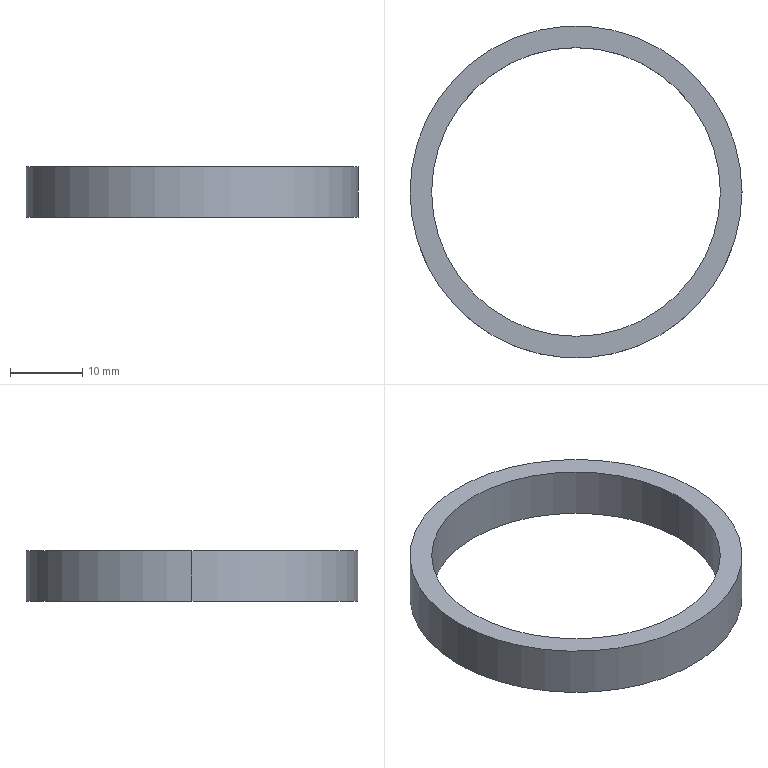Part | SolidWorks | features Extrusion 1 | 1 solid | 6 faces | box 46 x 46 x 7 mm | volume 2837 mm3 | cylinder 4 | plane 2 | commonest cylinder face diameters 40 x2 46 x2
STEP:
#1=CARTESIAN_POINT('',(-20.,0.,7.));
#2=VERTEX_POINT('',#1);
#3=CARTESIAN_POINT('',(20.,0.,7.));
#4=VERTEX_POINT('',#3);
#5=CARTESIAN_POINT('',(0.,0.,7.));
#6=DIRECTION('',(0.,0.,1.));
#7=DIRECTION('',(1.,0.,0.));
#8=AXIS2_PLACEMENT_3D('',#5,#6,#7);
#9=CIRCLE('',#8,20.);
#10=EDGE_CURVE('',#2,#4,#9,.T.);
#11=ORIENTED_EDGE('',*,*,#10,.T.);
#12=CARTESIAN_POINT('',(20.,0.,0.));
#13=VERTEX_POINT('',#12);
#14=CARTESIAN_POINT('',(20.,0.,7.));
#15=DIRECTION('',(0.,0.,-1.));
#16=VECTOR('',#15,1000.);
#17=LINE('',#14,#16);
#18=EDGE_CURVE('',#4,#13,#17,.T.);
#19=ORIENTED_EDGE('',*,*,#18,.T.);
#20=CARTESIAN_POINT('',(-20.,0.,0.));
#21=VERTEX_POINT('',#20);
#22=CARTESIAN_POINT('',(0.,0.,0.));
#23=DIRECTION('',(0.,0.,1.));
#24=DIRECTION('',(1.,0.,0.));
#25=AXIS2_PLACEMENT_3D('',#22,#23,#24);
#26=CIRCLE('',#25,20.);
#27=EDGE_CURVE('',#21,#13,#26,.T.);
#28=ORIENTED_EDGE('',*,*,#27,.F.);
#29=CARTESIAN_POINT('',(-20.,0.,7.));
#30=DIRECTION('',(0.,0.,-1.));
#31=VECTOR('',#30,1000.);
#32=LINE('',#29,#31);
#33=EDGE_CURVE('',#2,#21,#32,.T.);
#34=ORIENTED_EDGE('',*,*,#33,.F.);
#35=EDGE_LOOP('',(#11,#19,#28,#34));
#36=FACE_OUTER_BOUND('',#35,.T.);
#37=CARTESIAN_POINT('',(0.,0.,7.));
#38=DIRECTION('',(0.,0.,-1.));
#39=DIRECTION('',(-1.,0.,0.));
#40=AXIS2_PLACEMENT_3D('',#37,#38,#39);
#41=CYLINDRICAL_SURFACE('',#40,20.);
#42=ADVANCED_FACE('',(#36),#41,.F.);
#43=CARTESIAN_POINT('',(23.,0.,7.));
#44=VERTEX_POINT('',#43);
#45=CARTESIAN_POINT('',(-23.,0.,7.));
#46=VERTEX_POINT('',#45);
#47=CARTESIAN_POINT('',(0.,0.,7.));
#48=DIRECTION('',(0.,0.,1.));
#49=DIRECTION('',(1.,0.,0.));
#50=AXIS2_PLACEMENT_3D('',#47,#48,#49);
#51=CIRCLE('',#50,23.);
#52=EDGE_CURVE('',#44,#46,#51,.T.);
#53=ORIENTED_EDGE('',*,*,#52,.F.);
#54=CARTESIAN_POINT('',(23.,0.,0.));
#55=VERTEX_POINT('',#54);
#56=CARTESIAN_POINT('',(23.,0.,7.));
#57=DIRECTION('',(0.,0.,-1.));
#58=VECTOR('',#57,1000.);
#59=LINE('',#56,#58);
#60=EDGE_CURVE('',#44,#55,#59,.T.);
#61=ORIENTED_EDGE('',*,*,#60,.T.);
#62=CARTESIAN_POINT('',(-23.,0.,0.));
#63=VERTEX_POINT('',#62);
#64=CARTESIAN_POINT('',(0.,0.,0.));
#65=DIRECTION('',(0.,0.,1.));
#66=DIRECTION('',(1.,0.,0.));
#67=AXIS2_PLACEMENT_3D('',#64,#65,#66);
#68=CIRCLE('',#67,23.);
#69=EDGE_CURVE('',#55,#63,#68,.T.);
#70=ORIENTED_EDGE('',*,*,#69,.T.);
#71=CARTESIAN_POINT('',(-23.,0.,7.));
#72=DIRECTION('',(0.,0.,-1.));
#73=VECTOR('',#72,1000.);
#74=LINE('',#71,#73);
#75=EDGE_CURVE('',#46,#63,#74,.T.);
#76=ORIENTED_EDGE('',*,*,#75,.F.);
#77=EDGE_LOOP('',(#53,#61,#70,#76));
#78=FACE_OUTER_BOUND('',#77,.T.);
#79=CARTESIAN_POINT('',(0.,0.,7.));
#80=DIRECTION('',(0.,0.,-1.));
#81=DIRECTION('',(-1.,0.,0.));
#82=AXIS2_PLACEMENT_3D('',#79,#80,#81);
#83=CYLINDRICAL_SURFACE('',#82,23.);
#84=ADVANCED_FACE('',(#78),#83,.T.);
#85=CARTESIAN_POINT('',(0.,0.,7.));
#86=DIRECTION('',(0.,0.,1.));
#87=DIRECTION('',(1.,0.,0.));
#88=AXIS2_PLACEMENT_3D('',#85,#86,#87);
#89=CIRCLE('',#88,23.);
#90=EDGE_CURVE('',#46,#44,#89,.T.);
#91=ORIENTED_EDGE('',*,*,#90,.T.);
#92=ORIENTED_EDGE('',*,*,#52,.T.);
#93=EDGE_LOOP('',(#91,#92));
#94=FACE_OUTER_BOUND('',#93,.T.);
#95=ORIENTED_EDGE('',*,*,#10,.F.);
#96=CARTESIAN_POINT('',(0.,0.,7.));
#97=DIRECTION('',(0.,0.,1.));
#98=DIRECTION('',(1.,0.,0.));
#99=AXIS2_PLACEMENT_3D('',#96,#97,#98);
#100=CIRCLE('',#99,20.);
#101=EDGE_CURVE('',#4,#2,#100,.T.);
#102=ORIENTED_EDGE('',*,*,#101,.F.);
#103=EDGE_LOOP('',(#95,#102));
#104=FACE_BOUND('',#103,.T.);
#105=CARTESIAN_POINT('',(0.,0.,7.));
#106=DIRECTION('',(0.,0.,1.));
#107=DIRECTION('',(1.,0.,0.));
#108=AXIS2_PLACEMENT_3D('',#105,#106,#107);
#109=PLANE('',#108);
#110=ADVANCED_FACE('',(#94,#104),#109,.T.);
#111=CARTESIAN_POINT('',(0.,0.,0.));
#112=DIRECTION('',(0.,0.,1.));
#113=DIRECTION('',(1.,0.,0.));
#114=AXIS2_PLACEMENT_3D('',#111,#112,#113);
#115=CIRCLE('',#114,23.);
#116=EDGE_CURVE('',#63,#55,#115,.T.);
#117=ORIENTED_EDGE('',*,*,#116,.F.);
#118=ORIENTED_EDGE('',*,*,#69,.F.);
#119=EDGE_LOOP('',(#117,#118));
#120=FACE_OUTER_BOUND('',#119,.T.);
#121=ORIENTED_EDGE('',*,*,#27,.T.);
#122=CARTESIAN_POINT('',(0.,0.,0.));
#123=DIRECTION('',(0.,0.,1.));
#124=DIRECTION('',(1.,0.,0.));
#125=AXIS2_PLACEMENT_3D('',#122,#123,#124);
#126=CIRCLE('',#125,20.);
#127=EDGE_CURVE('',#13,#21,#126,.T.);
#128=ORIENTED_EDGE('',*,*,#127,.T.);
#129=EDGE_LOOP('',(#121,#128));
#130=FACE_BOUND('',#129,.T.);
#131=CARTESIAN_POINT('',(0.,0.,0.));
#132=DIRECTION('',(0.,0.,1.));
#133=DIRECTION('',(1.,0.,0.));
#134=AXIS2_PLACEMENT_3D('',#131,#132,#133);
#135=PLANE('',#134);
#136=ADVANCED_FACE('',(#120,#130),#135,.F.);
#137=ORIENTED_EDGE('',*,*,#60,.F.);
#138=ORIENTED_EDGE('',*,*,#90,.F.);
#139=ORIENTED_EDGE('',*,*,#75,.T.);
#140=ORIENTED_EDGE('',*,*,#116,.T.);
#141=EDGE_LOOP('',(#137,#138,#139,#140));
#142=FACE_OUTER_BOUND('',#141,.T.);
#143=CARTESIAN_POINT('',(0.,0.,7.));
#144=DIRECTION('',(0.,0.,-1.));
#145=DIRECTION('',(-1.,0.,0.));
#146=AXIS2_PLACEMENT_3D('',#143,#144,#145);
#147=CYLINDRICAL_SURFACE('',#146,23.);
#148=ADVANCED_FACE('',(#142),#147,.T.);
#149=ORIENTED_EDGE('',*,*,#18,.F.);
#150=ORIENTED_EDGE('',*,*,#101,.T.);
#151=ORIENTED_EDGE('',*,*,#33,.T.);
#152=ORIENTED_EDGE('',*,*,#127,.F.);
#153=EDGE_LOOP('',(#149,#150,#151,#152));
#154=FACE_OUTER_BOUND('',#153,.T.);
#155=CARTESIAN_POINT('',(0.,0.,7.));
#156=DIRECTION('',(0.,0.,-1.));
#157=DIRECTION('',(-1.,0.,0.));
#158=AXIS2_PLACEMENT_3D('',#155,#156,#157);
#159=CYLINDRICAL_SURFACE('',#158,20.);
#160=ADVANCED_FACE('',(#154),#159,.F.);
#161=CLOSED_SHELL('',(#42,#84,#110,#136,#148,#160));
#162=MANIFOLD_SOLID_BREP('',#161);
#163=CARTESIAN_POINT('',(0.,0.,0.));
#164=DIRECTION('',(0.,0.,1.));
#165=DIRECTION('',(1.,0.,0.));
#166=AXIS2_PLACEMENT_3D('',#163,#164,#165);
#167=(LENGTH_UNIT()NAMED_UNIT(*)SI_UNIT(.MILLI.,.METRE.));
#168=UNCERTAINTY_MEASURE_WITH_UNIT(LENGTH_MEASURE(0.00001),#167,'','');
#169=(NAMED_UNIT(*)PLANE_ANGLE_UNIT()SI_UNIT($,.RADIAN.));
#170=(NAMED_UNIT(*)SI_UNIT($,.STERADIAN.)SOLID_ANGLE_UNIT());
#171=(GEOMETRIC_REPRESENTATION_CONTEXT(3)GLOBAL_UNCERTAINTY_ASSIGNED_CONTEXT((#168))GLOBAL_UNIT_ASSIGNED_CONTEXT((#167,#169,#170))REPRESENTATION_CONTEXT('',''));
#172=ADVANCED_BREP_SHAPE_REPRESENTATION('',(#162,#166),#171);